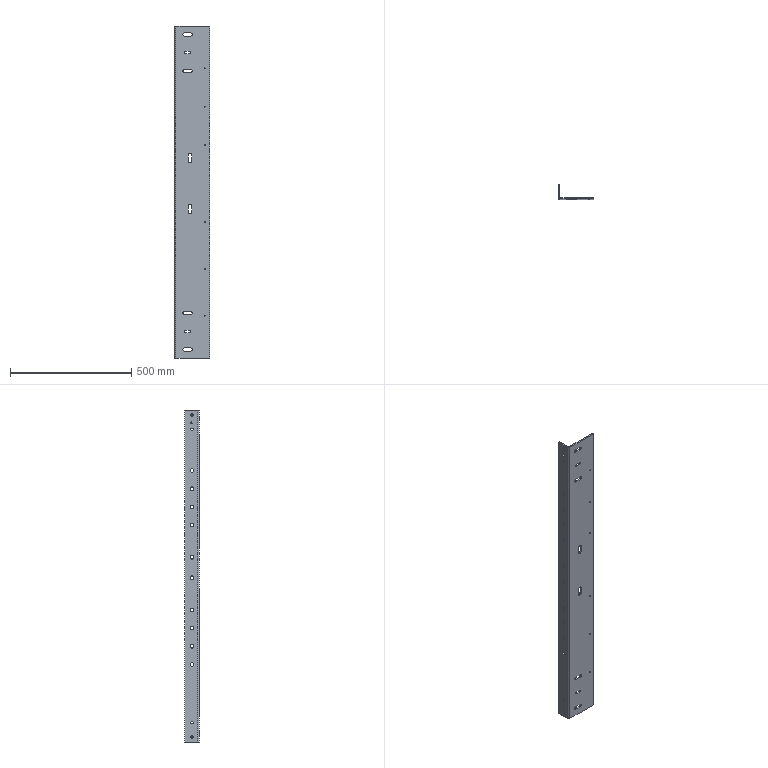Part | SolidWorks | features ICE 3, Cut 1, EdgeFlange 1, FlatPattern 1, SMBaseFlange 1, SheetMetal 1 | 1 solid | 91 faces | box 145 x 60 x 1370 mm | volume 1590981 mm3 | cylinder 60 | plane 31 | commonest cylinder face diameters 15 x20 4.5 x12 10 x8 13 x8 14 x6 11 x4